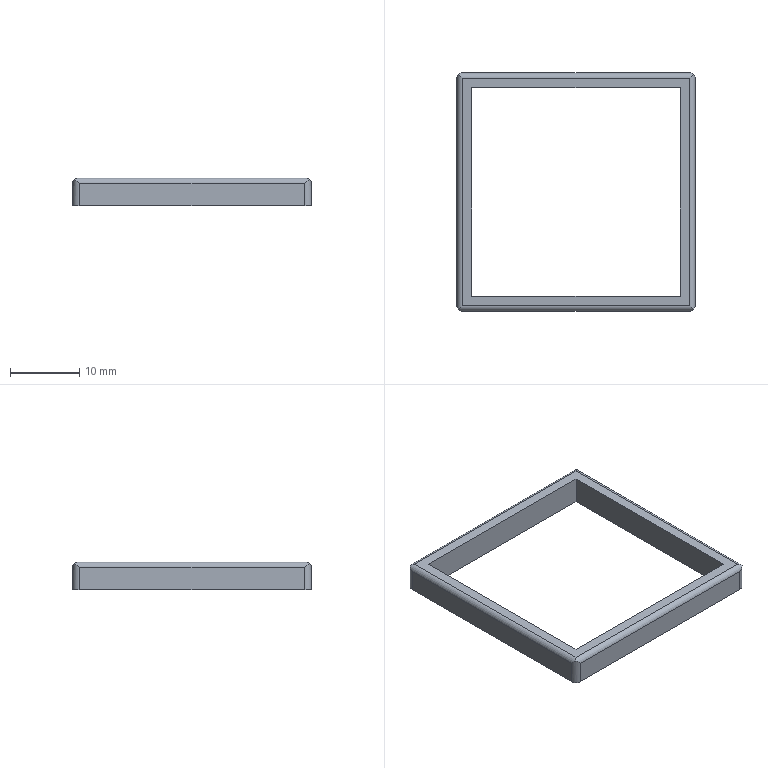Part | NX | 1 solid | 18 faces | box 34.5 x 34.5 x 4 mm | volume 1113 mm3 | plane 10 | cylinder 8 | commonest cylinder face diameters 1.6 x4 2 x4
STEP:
#1=CARTESIAN_POINT('',(16.45,-16.45,21.8));
#2=VERTEX_POINT('',#1);
#3=CARTESIAN_POINT('',(16.957,-16.957,21.619));
#4=VERTEX_POINT('',#3);
#5=CARTESIAN_POINT('',(16.45,-16.45,21.));
#6=DIRECTION('',(-0.7071,-0.7071,0.));
#7=DIRECTION('',(-0.7071,0.7071,0.));
#8=AXIS2_PLACEMENT_3D('',#5,#6,#7);
#9=ELLIPSE('',#8,1.131,0.8);
#10=EDGE_CURVE('',#2,#4,#9,.F.);
#11=ORIENTED_EDGE('',*,*,#10,.F.);
#12=CARTESIAN_POINT('',(-16.45,-16.45,21.8));
#13=VERTEX_POINT('',#12);
#14=CARTESIAN_POINT('',(17.25,-16.45,21.8));
#15=DIRECTION('',(-1.,0.,0.));
#16=VECTOR('',#15,1000.);
#17=LINE('',#14,#16);
#18=EDGE_CURVE('',#2,#13,#17,.T.);
#19=ORIENTED_EDGE('',*,*,#18,.T.);
#20=CARTESIAN_POINT('',(-16.957,-16.957,21.619));
#21=VERTEX_POINT('',#20);
#22=CARTESIAN_POINT('',(-16.45,-16.45,21.));
#23=DIRECTION('',(-0.7071,0.7071,0.));
#24=DIRECTION('',(-0.7071,-0.7071,0.));
#25=AXIS2_PLACEMENT_3D('',#22,#23,#24);
#26=ELLIPSE('',#25,1.131,0.8);
#27=EDGE_CURVE('',#21,#13,#26,.T.);
#28=ORIENTED_EDGE('',*,*,#27,.F.);
#29=CARTESIAN_POINT('',(-16.25,-17.25,21.));
#30=VERTEX_POINT('',#29);
#31=CARTESIAN_POINT('',(-16.957,-16.957,21.619));
#32=CARTESIAN_POINT('',(-16.753,-17.161,21.452));
#33=CARTESIAN_POINT('',(-16.498,-17.25,21.222));
#34=CARTESIAN_POINT('',(-16.25,-17.25,21.));
#35=B_SPLINE_CURVE_WITH_KNOTS('',3,(#31,#32,#33,#34),.UNSPECIFIED.,.F.,.F.,(4,4),(0.0006147,0.001614),.UNSPECIFIED.);
#36=EDGE_CURVE('',#30,#21,#35,.F.);
#37=ORIENTED_EDGE('',*,*,#36,.F.);
#38=CARTESIAN_POINT('',(16.25,-17.25,21.));
#39=VERTEX_POINT('',#38);
#40=CARTESIAN_POINT('',(17.25,-17.25,21.));
#41=DIRECTION('',(-1.,0.,0.));
#42=VECTOR('',#41,1000.);
#43=LINE('',#40,#42);
#44=EDGE_CURVE('',#39,#30,#43,.T.);
#45=ORIENTED_EDGE('',*,*,#44,.F.);
#46=CARTESIAN_POINT('',(16.957,-16.957,21.619));
#47=CARTESIAN_POINT('',(16.753,-17.161,21.452));
#48=CARTESIAN_POINT('',(16.498,-17.25,21.222));
#49=CARTESIAN_POINT('',(16.25,-17.25,21.));
#50=B_SPLINE_CURVE_WITH_KNOTS('',3,(#46,#47,#48,#49),.UNSPECIFIED.,.F.,.F.,(4,4),(0.0006147,0.001614),.UNSPECIFIED.);
#51=EDGE_CURVE('',#4,#39,#50,.T.);
#52=ORIENTED_EDGE('',*,*,#51,.F.);
#53=EDGE_LOOP('',(#11,#19,#28,#37,#45,#52));
#54=FACE_BOUND('',#53,.T.);
#55=CARTESIAN_POINT('',(17.25,-16.45,21.));
#56=DIRECTION('',(-1.,0.,0.));
#57=DIRECTION('',(0.,0.,1.));
#58=AXIS2_PLACEMENT_3D('',#55,#56,#57);
#59=CYLINDRICAL_SURFACE('',#58,0.8);
#60=ADVANCED_FACE('',(#54),#59,.T.);
#61=CARTESIAN_POINT('',(16.957,16.957,21.619));
#62=VERTEX_POINT('',#61);
#63=CARTESIAN_POINT('',(16.45,16.45,21.8));
#64=VERTEX_POINT('',#63);
#65=CARTESIAN_POINT('',(16.45,16.45,21.));
#66=DIRECTION('',(-0.7071,0.7071,0.));
#67=DIRECTION('',(-0.7071,-0.7071,0.));
#68=AXIS2_PLACEMENT_3D('',#65,#66,#67);
#69=ELLIPSE('',#68,1.131,0.8);
#70=EDGE_CURVE('',#62,#64,#69,.F.);
#71=ORIENTED_EDGE('',*,*,#70,.F.);
#72=CARTESIAN_POINT('',(16.25,17.25,21.));
#73=VERTEX_POINT('',#72);
#74=CARTESIAN_POINT('',(16.957,16.957,21.619));
#75=CARTESIAN_POINT('',(16.753,17.161,21.452));
#76=CARTESIAN_POINT('',(16.498,17.25,21.222));
#77=CARTESIAN_POINT('',(16.25,17.25,21.));
#78=B_SPLINE_CURVE_WITH_KNOTS('',3,(#74,#75,#76,#77),.UNSPECIFIED.,.F.,.F.,(4,4),(0.0006147,0.001614),.UNSPECIFIED.);
#79=EDGE_CURVE('',#73,#62,#78,.F.);
#80=ORIENTED_EDGE('',*,*,#79,.F.);
#81=CARTESIAN_POINT('',(-16.25,17.25,21.));
#82=VERTEX_POINT('',#81);
#83=CARTESIAN_POINT('',(17.25,17.25,21.));
#84=DIRECTION('',(-1.,0.,0.));
#85=VECTOR('',#84,1000.);
#86=LINE('',#83,#85);
#87=EDGE_CURVE('',#73,#82,#86,.T.);
#88=ORIENTED_EDGE('',*,*,#87,.T.);
#89=CARTESIAN_POINT('',(-16.957,16.957,21.619));
#90=VERTEX_POINT('',#89);
#91=CARTESIAN_POINT('',(-16.957,16.957,21.619));
#92=CARTESIAN_POINT('',(-16.753,17.161,21.452));
#93=CARTESIAN_POINT('',(-16.498,17.25,21.222));
#94=CARTESIAN_POINT('',(-16.25,17.25,21.));
#95=B_SPLINE_CURVE_WITH_KNOTS('',3,(#91,#92,#93,#94),.UNSPECIFIED.,.F.,.F.,(4,4),(0.0006147,0.001614),.UNSPECIFIED.);
#96=EDGE_CURVE('',#90,#82,#95,.T.);
#97=ORIENTED_EDGE('',*,*,#96,.F.);
#98=CARTESIAN_POINT('',(-16.45,16.45,21.8));
#99=VERTEX_POINT('',#98);
#100=CARTESIAN_POINT('',(-16.45,16.45,21.));
#101=DIRECTION('',(-0.7071,-0.7071,0.));
#102=DIRECTION('',(-0.7071,0.7071,0.));
#103=AXIS2_PLACEMENT_3D('',#100,#101,#102);
#104=ELLIPSE('',#103,1.131,0.8);
#105=EDGE_CURVE('',#99,#90,#104,.T.);
#106=ORIENTED_EDGE('',*,*,#105,.F.);
#107=CARTESIAN_POINT('',(17.25,16.45,21.8));
#108=DIRECTION('',(-1.,0.,0.));
#109=VECTOR('',#108,1000.);
#110=LINE('',#107,#109);
#111=EDGE_CURVE('',#64,#99,#110,.T.);
#112=ORIENTED_EDGE('',*,*,#111,.F.);
#113=EDGE_LOOP('',(#71,#80,#88,#97,#106,#112));
#114=FACE_BOUND('',#113,.T.);
#115=CARTESIAN_POINT('',(17.25,16.45,21.));
#116=DIRECTION('',(-1.,0.,0.));
#117=DIRECTION('',(0.,0.,1.));
#118=AXIS2_PLACEMENT_3D('',#115,#116,#117);
#119=CYLINDRICAL_SURFACE('',#118,0.8);
#120=ADVANCED_FACE('',(#114),#119,.T.);
#121=CARTESIAN_POINT('',(-15.05,-15.05,21.8));
#122=VERTEX_POINT('',#121);
#123=CARTESIAN_POINT('',(-15.05,15.05,21.8));
#124=VERTEX_POINT('',#123);
#125=CARTESIAN_POINT('',(-15.05,16.45,21.8));
#126=DIRECTION('',(0.,1.,0.));
#127=VECTOR('',#126,1000.);
#128=LINE('',#125,#127);
#129=EDGE_CURVE('',#122,#124,#128,.T.);
#130=ORIENTED_EDGE('',*,*,#129,.T.);
#131=CARTESIAN_POINT('',(15.05,15.05,21.8));
#132=VERTEX_POINT('',#131);
#133=CARTESIAN_POINT('',(17.25,15.05,21.8));
#134=DIRECTION('',(1.,0.,0.));
#135=VECTOR('',#134,1000.);
#136=LINE('',#133,#135);
#137=EDGE_CURVE('',#124,#132,#136,.T.);
#138=ORIENTED_EDGE('',*,*,#137,.T.);
#139=CARTESIAN_POINT('',(15.05,-15.05,21.8));
#140=VERTEX_POINT('',#139);
#141=CARTESIAN_POINT('',(15.05,16.45,21.8));
#142=DIRECTION('',(0.,-1.,0.));
#143=VECTOR('',#142,1000.);
#144=LINE('',#141,#143);
#145=EDGE_CURVE('',#132,#140,#144,.T.);
#146=ORIENTED_EDGE('',*,*,#145,.T.);
#147=CARTESIAN_POINT('',(17.25,-15.05,21.8));
#148=DIRECTION('',(-1.,0.,0.));
#149=VECTOR('',#148,1000.);
#150=LINE('',#147,#149);
#151=EDGE_CURVE('',#140,#122,#150,.T.);
#152=ORIENTED_EDGE('',*,*,#151,.T.);
#153=EDGE_LOOP('',(#130,#138,#146,#152));
#154=FACE_BOUND('',#153,.T.);
#155=ORIENTED_EDGE('',*,*,#18,.F.);
#156=CARTESIAN_POINT('',(16.45,-17.25,21.8));
#157=DIRECTION('',(0.,1.,0.));
#158=VECTOR('',#157,1000.);
#159=LINE('',#156,#158);
#160=EDGE_CURVE('',#2,#64,#159,.T.);
#161=ORIENTED_EDGE('',*,*,#160,.T.);
#162=ORIENTED_EDGE('',*,*,#111,.T.);
#163=CARTESIAN_POINT('',(-16.45,-17.25,21.8));
#164=DIRECTION('',(0.,1.,0.));
#165=VECTOR('',#164,1000.);
#166=LINE('',#163,#165);
#167=EDGE_CURVE('',#13,#99,#166,.T.);
#168=ORIENTED_EDGE('',*,*,#167,.F.);
#169=EDGE_LOOP('',(#155,#161,#162,#168));
#170=FACE_BOUND('',#169,.T.);
#171=CARTESIAN_POINT('',(17.25,16.45,21.8));
#172=DIRECTION('',(0.,0.,-1.));
#173=DIRECTION('',(-1.,0.,0.));
#174=AXIS2_PLACEMENT_3D('',#171,#172,#173);
#175=PLANE('',#174);
#176=ADVANCED_FACE('',(#154,#170),#175,.F.);
#177=CARTESIAN_POINT('',(-17.25,16.25,17.8));
#178=VERTEX_POINT('',#177);
#179=CARTESIAN_POINT('',(-17.25,16.25,21.));
#180=VERTEX_POINT('',#179);
#181=CARTESIAN_POINT('',(-17.25,16.25,17.8));
#182=DIRECTION('',(0.,0.,1.));
#183=VECTOR('',#182,1000.);
#184=LINE('',#181,#183);
#185=EDGE_CURVE('',#178,#180,#184,.T.);
#186=ORIENTED_EDGE('',*,*,#185,.T.);
#187=CARTESIAN_POINT('',(-16.957,16.957,21.619));
#188=CARTESIAN_POINT('',(-17.161,16.753,21.452));
#189=CARTESIAN_POINT('',(-17.25,16.498,21.222));
#190=CARTESIAN_POINT('',(-17.25,16.25,21.));
#191=B_SPLINE_CURVE_WITH_KNOTS('',3,(#187,#188,#189,#190),.UNSPECIFIED.,.F.,.F.,(4,4),(0.0006147,0.001614),.UNSPECIFIED.);
#192=EDGE_CURVE('',#180,#90,#191,.F.);
#193=ORIENTED_EDGE('',*,*,#192,.T.);
#194=ORIENTED_EDGE('',*,*,#96,.T.);
#195=CARTESIAN_POINT('',(-16.25,17.25,17.8));
#196=VERTEX_POINT('',#195);
#197=CARTESIAN_POINT('',(-16.25,17.25,17.8));
#198=DIRECTION('',(0.,0.,1.));
#199=VECTOR('',#198,1000.);
#200=LINE('',#197,#199);
#201=EDGE_CURVE('',#196,#82,#200,.T.);
#202=ORIENTED_EDGE('',*,*,#201,.F.);
#203=CARTESIAN_POINT('',(-16.25,16.25,17.8));
#204=DIRECTION('',(0.,0.,1.));
#205=DIRECTION('',(1.,0.,0.));
#206=AXIS2_PLACEMENT_3D('',#203,#204,#205);
#207=CIRCLE('',#206,1.);
#208=EDGE_CURVE('',#196,#178,#207,.T.);
#209=ORIENTED_EDGE('',*,*,#208,.T.);
#210=EDGE_LOOP('',(#186,#193,#194,#202,#209));
#211=FACE_BOUND('',#210,.T.);
#212=CARTESIAN_POINT('',(-16.25,16.25,17.8));
#213=DIRECTION('',(0.,0.,1.));
#214=DIRECTION('',(1.,0.,0.));
#215=AXIS2_PLACEMENT_3D('',#212,#213,#214);
#216=CYLINDRICAL_SURFACE('',#215,1.);
#217=ADVANCED_FACE('',(#211),#216,.T.);
#218=ORIENTED_EDGE('',*,*,#36,.T.);
#219=CARTESIAN_POINT('',(-17.25,-16.25,21.));
#220=VERTEX_POINT('',#219);
#221=CARTESIAN_POINT('',(-16.957,-16.957,21.619));
#222=CARTESIAN_POINT('',(-17.161,-16.753,21.452));
#223=CARTESIAN_POINT('',(-17.25,-16.498,21.222));
#224=CARTESIAN_POINT('',(-17.25,-16.25,21.));
#225=B_SPLINE_CURVE_WITH_KNOTS('',3,(#221,#222,#223,#224),.UNSPECIFIED.,.F.,.F.,(4,4),(0.0006147,0.001614),.UNSPECIFIED.);
#226=EDGE_CURVE('',#21,#220,#225,.T.);
#227=ORIENTED_EDGE('',*,*,#226,.T.);
#228=CARTESIAN_POINT('',(-17.25,-16.25,17.8));
#229=VERTEX_POINT('',#228);
#230=CARTESIAN_POINT('',(-17.25,-16.25,17.8));
#231=DIRECTION('',(0.,0.,1.));
#232=VECTOR('',#231,1000.);
#233=LINE('',#230,#232);
#234=EDGE_CURVE('',#229,#220,#233,.T.);
#235=ORIENTED_EDGE('',*,*,#234,.F.);
#236=CARTESIAN_POINT('',(-16.25,-17.25,17.8));
#237=VERTEX_POINT('',#236);
#238=CARTESIAN_POINT('',(-16.25,-16.25,17.8));
#239=DIRECTION('',(0.,0.,1.));
#240=DIRECTION('',(1.,0.,0.));
#241=AXIS2_PLACEMENT_3D('',#238,#239,#240);
#242=CIRCLE('',#241,1.);
#243=EDGE_CURVE('',#229,#237,#242,.T.);
#244=ORIENTED_EDGE('',*,*,#243,.T.);
#245=CARTESIAN_POINT('',(-16.25,-17.25,17.8));
#246=DIRECTION('',(0.,0.,1.));
#247=VECTOR('',#246,1000.);
#248=LINE('',#245,#247);
#249=EDGE_CURVE('',#237,#30,#248,.T.);
#250=ORIENTED_EDGE('',*,*,#249,.T.);
#251=EDGE_LOOP('',(#218,#227,#235,#244,#250));
#252=FACE_BOUND('',#251,.T.);
#253=CARTESIAN_POINT('',(-16.25,-16.25,17.8));
#254=DIRECTION('',(0.,0.,1.));
#255=DIRECTION('',(1.,0.,0.));
#256=AXIS2_PLACEMENT_3D('',#253,#254,#255);
#257=CYLINDRICAL_SURFACE('',#256,1.);
#258=ADVANCED_FACE('',(#252),#257,.T.);
#259=CARTESIAN_POINT('',(17.25,-16.25,17.8));
#260=VERTEX_POINT('',#259);
#261=CARTESIAN_POINT('',(17.25,-16.25,21.));
#262=VERTEX_POINT('',#261);
#263=CARTESIAN_POINT('',(17.25,-16.25,17.8));
#264=DIRECTION('',(0.,0.,1.));
#265=VECTOR('',#264,1000.);
#266=LINE('',#263,#265);
#267=EDGE_CURVE('',#260,#262,#266,.T.);
#268=ORIENTED_EDGE('',*,*,#267,.T.);
#269=CARTESIAN_POINT('',(16.957,-16.957,21.619));
#270=CARTESIAN_POINT('',(17.161,-16.753,21.452));
#271=CARTESIAN_POINT('',(17.25,-16.498,21.222));
#272=CARTESIAN_POINT('',(17.25,-16.25,21.));
#273=B_SPLINE_CURVE_WITH_KNOTS('',3,(#269,#270,#271,#272),.UNSPECIFIED.,.F.,.F.,(4,4),(0.0006147,0.001614),.UNSPECIFIED.);
#274=EDGE_CURVE('',#262,#4,#273,.F.);
#275=ORIENTED_EDGE('',*,*,#274,.T.);
#276=ORIENTED_EDGE('',*,*,#51,.T.);
#277=CARTESIAN_POINT('',(16.25,-17.25,17.8));
#278=VERTEX_POINT('',#277);
#279=CARTESIAN_POINT('',(16.25,-17.25,17.8));
#280=DIRECTION('',(0.,0.,1.));
#281=VECTOR('',#280,1000.);
#282=LINE('',#279,#281);
#283=EDGE_CURVE('',#278,#39,#282,.T.);
#284=ORIENTED_EDGE('',*,*,#283,.F.);
#285=CARTESIAN_POINT('',(16.25,-16.25,17.8));
#286=DIRECTION('',(0.,0.,1.));
#287=DIRECTION('',(1.,0.,0.));
#288=AXIS2_PLACEMENT_3D('',#285,#286,#287);
#289=CIRCLE('',#288,1.);
#290=EDGE_CURVE('',#278,#260,#289,.T.);
#291=ORIENTED_EDGE('',*,*,#290,.T.);
#292=EDGE_LOOP('',(#268,#275,#276,#284,#291));
#293=FACE_BOUND('',#292,.T.);
#294=CARTESIAN_POINT('',(16.25,-16.25,17.8));
#295=DIRECTION('',(0.,0.,1.));
#296=DIRECTION('',(1.,0.,0.));
#297=AXIS2_PLACEMENT_3D('',#294,#295,#296);
#298=CYLINDRICAL_SURFACE('',#297,1.);
#299=ADVANCED_FACE('',(#293),#298,.T.);
#300=ORIENTED_EDGE('',*,*,#79,.T.);
#301=CARTESIAN_POINT('',(17.25,16.25,21.));
#302=VERTEX_POINT('',#301);
#303=CARTESIAN_POINT('',(16.957,16.957,21.619));
#304=CARTESIAN_POINT('',(17.161,16.753,21.452));
#305=CARTESIAN_POINT('',(17.25,16.498,21.222));
#306=CARTESIAN_POINT('',(17.25,16.25,21.));
#307=B_SPLINE_CURVE_WITH_KNOTS('',3,(#303,#304,#305,#306),.UNSPECIFIED.,.F.,.F.,(4,4),(0.0006147,0.001614),.UNSPECIFIED.);
#308=EDGE_CURVE('',#62,#302,#307,.T.);
#309=ORIENTED_EDGE('',*,*,#308,.T.);
#310=CARTESIAN_POINT('',(17.25,16.25,17.8));
#311=VERTEX_POINT('',#310);
#312=CARTESIAN_POINT('',(17.25,16.25,17.8));
#313=DIRECTION('',(0.,0.,1.));
#314=VECTOR('',#313,1000.);
#315=LINE('',#312,#314);
#316=EDGE_CURVE('',#311,#302,#315,.T.);
#317=ORIENTED_EDGE('',*,*,#316,.F.);
#318=CARTESIAN_POINT('',(16.25,17.25,17.8));
#319=VERTEX_POINT('',#318);
#320=CARTESIAN_POINT('',(16.25,16.25,17.8));
#321=DIRECTION('',(0.,0.,1.));
#322=DIRECTION('',(1.,0.,0.));
#323=AXIS2_PLACEMENT_3D('',#320,#321,#322);
#324=CIRCLE('',#323,1.);
#325=EDGE_CURVE('',#311,#319,#324,.T.);
#326=ORIENTED_EDGE('',*,*,#325,.T.);
#327=CARTESIAN_POINT('',(16.25,17.25,17.8));
#328=DIRECTION('',(0.,0.,1.));
#329=VECTOR('',#328,1000.);
#330=LINE('',#327,#329);
#331=EDGE_CURVE('',#319,#73,#330,.T.);
#332=ORIENTED_EDGE('',*,*,#331,.T.);
#333=EDGE_LOOP('',(#300,#309,#317,#326,#332));
#334=FACE_BOUND('',#333,.T.);
#335=CARTESIAN_POINT('',(16.25,16.25,17.8));
#336=DIRECTION('',(0.,0.,1.));
#337=DIRECTION('',(1.,0.,0.));
#338=AXIS2_PLACEMENT_3D('',#335,#336,#337);
#339=CYLINDRICAL_SURFACE('',#338,1.);
#340=ADVANCED_FACE('',(#334),#339,.T.);
#341=ORIENTED_EDGE('',*,*,#249,.F.);
#342=CARTESIAN_POINT('',(17.25,-17.25,17.8));
#343=DIRECTION('',(-1.,0.,0.));
#344=VECTOR('',#343,1000.);
#345=LINE('',#342,#344);
#346=EDGE_CURVE('',#278,#237,#345,.T.);
#347=ORIENTED_EDGE('',*,*,#346,.F.);
#348=ORIENTED_EDGE('',*,*,#283,.T.);
#349=ORIENTED_EDGE('',*,*,#44,.T.);
#350=EDGE_LOOP('',(#341,#347,#348,#349));
#351=FACE_BOUND('',#350,.T.);
#352=CARTESIAN_POINT('',(17.25,-17.25,21.));
#353=DIRECTION('',(0.,1.,0.));
#354=DIRECTION('',(0.,0.,1.));
#355=AXIS2_PLACEMENT_3D('',#352,#353,#354);
#356=PLANE('',#355);
#357=ADVANCED_FACE('',(#351),#356,.F.);
#358=CARTESIAN_POINT('',(15.05,-15.05,17.8));
#359=VERTEX_POINT('',#358);
#360=CARTESIAN_POINT('',(15.05,15.05,17.8));
#361=VERTEX_POINT('',#360);
#362=CARTESIAN_POINT('',(15.05,-15.05,17.8));
#363=DIRECTION('',(0.,1.,0.));
#364=VECTOR('',#363,1000.);
#365=LINE('',#362,#364);
#366=EDGE_CURVE('',#359,#361,#365,.T.);
#367=ORIENTED_EDGE('',*,*,#366,.T.);
#368=CARTESIAN_POINT('',(-15.05,15.05,17.8));
#369=VERTEX_POINT('',#368);
#370=CARTESIAN_POINT('',(15.05,15.05,17.8));
#371=DIRECTION('',(-1.,0.,0.));
#372=VECTOR('',#371,1000.);
#373=LINE('',#370,#372);
#374=EDGE_CURVE('',#361,#369,#373,.T.);
#375=ORIENTED_EDGE('',*,*,#374,.T.);
#376=CARTESIAN_POINT('',(-15.05,-15.05,17.8));
#377=VERTEX_POINT('',#376);
#378=CARTESIAN_POINT('',(-15.05,15.05,17.8));
#379=DIRECTION('',(0.,-1.,0.));
#380=VECTOR('',#379,1000.);
#381=LINE('',#378,#380);
#382=EDGE_CURVE('',#369,#377,#381,.T.);
#383=ORIENTED_EDGE('',*,*,#382,.T.);
#384=CARTESIAN_POINT('',(-15.05,-15.05,17.8));
#385=DIRECTION('',(1.,0.,0.));
#386=VECTOR('',#385,1000.);
#387=LINE('',#384,#386);
#388=EDGE_CURVE('',#377,#359,#387,.T.);
#389=ORIENTED_EDGE('',*,*,#388,.T.);
#390=EDGE_LOOP('',(#367,#375,#383,#389));
#391=FACE_BOUND('',#390,.T.);
#392=ORIENTED_EDGE('',*,*,#243,.F.);
#393=CARTESIAN_POINT('',(-17.25,-17.25,17.8));
#394=DIRECTION('',(0.,1.,0.));
#395=VECTOR('',#394,1000.);
#396=LINE('',#393,#395);
#397=EDGE_CURVE('',#229,#178,#396,.T.);
#398=ORIENTED_EDGE('',*,*,#397,.T.);
#399=ORIENTED_EDGE('',*,*,#208,.F.);
#400=CARTESIAN_POINT('',(17.25,17.25,17.8));
#401=DIRECTION('',(-1.,0.,0.));
#402=VECTOR('',#401,1000.);
#403=LINE('',#400,#402);
#404=EDGE_CURVE('',#319,#196,#403,.T.);
#405=ORIENTED_EDGE('',*,*,#404,.F.);
#406=ORIENTED_EDGE('',*,*,#325,.F.);
#407=CARTESIAN_POINT('',(17.25,-17.25,17.8));
#408=DIRECTION('',(0.,1.,0.));
#409=VECTOR('',#408,1000.);
#410=LINE('',#407,#409);
#411=EDGE_CURVE('',#260,#311,#410,.T.);
#412=ORIENTED_EDGE('',*,*,#411,.F.);
#413=ORIENTED_EDGE('',*,*,#290,.F.);
#414=ORIENTED_EDGE('',*,*,#346,.T.);
#415=EDGE_LOOP('',(#392,#398,#399,#405,#406,#412,#413,#414));
#416=FACE_BOUND('',#415,.T.);
#417=CARTESIAN_POINT('',(17.25,-17.25,17.8));
#418=DIRECTION('',(0.,0.,1.));
#419=DIRECTION('',(1.,0.,0.));
#420=AXIS2_PLACEMENT_3D('',#417,#418,#419);
#421=PLANE('',#420);
#422=ADVANCED_FACE('',(#391,#416),#421,.F.);
#423=ORIENTED_EDGE('',*,*,#404,.T.);
#424=ORIENTED_EDGE('',*,*,#201,.T.);
#425=ORIENTED_EDGE('',*,*,#87,.F.);
#426=ORIENTED_EDGE('',*,*,#331,.F.);
#427=EDGE_LOOP('',(#423,#424,#425,#426));
#428=FACE_BOUND('',#427,.T.);
#429=CARTESIAN_POINT('',(17.25,17.25,17.8));
#430=DIRECTION('',(0.,-1.,0.));
#431=DIRECTION('',(0.,0.,-1.));
#432=AXIS2_PLACEMENT_3D('',#429,#430,#431);
#433=PLANE('',#432);
#434=ADVANCED_FACE('',(#428),#433,.F.);
#435=CARTESIAN_POINT('',(17.25,-17.25,21.));
#436=DIRECTION('',(0.,1.,0.));
#437=VECTOR('',#436,1000.);
#438=LINE('',#435,#437);
#439=EDGE_CURVE('',#262,#302,#438,.T.);
#440=ORIENTED_EDGE('',*,*,#439,.F.);
#441=ORIENTED_EDGE('',*,*,#267,.F.);
#442=ORIENTED_EDGE('',*,*,#411,.T.);
#443=ORIENTED_EDGE('',*,*,#316,.T.);
#444=EDGE_LOOP('',(#440,#441,#442,#443));
#445=FACE_BOUND('',#444,.T.);
#446=CARTESIAN_POINT('',(17.25,-16.45,21.));
#447=DIRECTION('',(1.,0.,0.));
#448=DIRECTION('',(0.,0.,-1.));
#449=AXIS2_PLACEMENT_3D('',#446,#447,#448);
#450=PLANE('',#449);
#451=ADVANCED_FACE('',(#445),#450,.T.);
#452=ORIENTED_EDGE('',*,*,#234,.T.);
#453=CARTESIAN_POINT('',(-17.25,-17.25,21.));
#454=DIRECTION('',(0.,1.,0.));
#455=VECTOR('',#454,1000.);
#456=LINE('',#453,#455);
#457=EDGE_CURVE('',#220,#180,#456,.T.);
#458=ORIENTED_EDGE('',*,*,#457,.T.);
#459=ORIENTED_EDGE('',*,*,#185,.F.);
#460=ORIENTED_EDGE('',*,*,#397,.F.);
#461=EDGE_LOOP('',(#452,#458,#459,#460));
#462=FACE_BOUND('',#461,.T.);
#463=CARTESIAN_POINT('',(-17.25,-16.45,21.));
#464=DIRECTION('',(1.,0.,0.));
#465=DIRECTION('',(0.,0.,-1.));
#466=AXIS2_PLACEMENT_3D('',#463,#464,#465);
#467=PLANE('',#466);
#468=ADVANCED_FACE('',(#462),#467,.F.);
#469=ORIENTED_EDGE('',*,*,#10,.T.);
#470=ORIENTED_EDGE('',*,*,#274,.F.);
#471=ORIENTED_EDGE('',*,*,#439,.T.);
#472=ORIENTED_EDGE('',*,*,#308,.F.);
#473=ORIENTED_EDGE('',*,*,#70,.T.);
#474=ORIENTED_EDGE('',*,*,#160,.F.);
#475=EDGE_LOOP('',(#469,#470,#471,#472,#473,#474));
#476=FACE_BOUND('',#475,.T.);
#477=CARTESIAN_POINT('',(16.45,-17.25,21.));
#478=DIRECTION('',(0.,1.,0.));
#479=DIRECTION('',(0.,0.,1.));
#480=AXIS2_PLACEMENT_3D('',#477,#478,#479);
#481=CYLINDRICAL_SURFACE('',#480,0.8);
#482=ADVANCED_FACE('',(#476),#481,.T.);
#483=ORIENTED_EDGE('',*,*,#105,.T.);
#484=ORIENTED_EDGE('',*,*,#192,.F.);
#485=ORIENTED_EDGE('',*,*,#457,.F.);
#486=ORIENTED_EDGE('',*,*,#226,.F.);
#487=ORIENTED_EDGE('',*,*,#27,.T.);
#488=ORIENTED_EDGE('',*,*,#167,.T.);
#489=EDGE_LOOP('',(#483,#484,#485,#486,#487,#488));
#490=FACE_BOUND('',#489,.T.);
#491=CARTESIAN_POINT('',(-16.45,-17.25,21.));
#492=DIRECTION('',(0.,1.,0.));
#493=DIRECTION('',(0.,0.,1.));
#494=AXIS2_PLACEMENT_3D('',#491,#492,#493);
#495=CYLINDRICAL_SURFACE('',#494,0.8);
#496=ADVANCED_FACE('',(#490),#495,.T.);
#497=CARTESIAN_POINT('',(-15.05,15.05,17.8));
#498=DIRECTION('',(0.,0.,1.));
#499=VECTOR('',#498,1000.);
#500=LINE('',#497,#499);
#501=EDGE_CURVE('',#369,#124,#500,.T.);
#502=ORIENTED_EDGE('',*,*,#501,.F.);
#503=ORIENTED_EDGE('',*,*,#374,.F.);
#504=CARTESIAN_POINT('',(15.05,15.05,17.8));
#505=DIRECTION('',(0.,0.,1.));
#506=VECTOR('',#505,1000.);
#507=LINE('',#504,#506);
#508=EDGE_CURVE('',#361,#132,#507,.T.);
#509=ORIENTED_EDGE('',*,*,#508,.T.);
#510=ORIENTED_EDGE('',*,*,#137,.F.);
#511=EDGE_LOOP('',(#502,#503,#509,#510));
#512=FACE_BOUND('',#511,.T.);
#513=CARTESIAN_POINT('',(15.05,15.05,17.8));
#514=DIRECTION('',(0.,1.,0.));
#515=DIRECTION('',(0.,0.,1.));
#516=AXIS2_PLACEMENT_3D('',#513,#514,#515);
#517=PLANE('',#516);
#518=ADVANCED_FACE('',(#512),#517,.F.);
#519=ORIENTED_EDGE('',*,*,#508,.F.);
#520=ORIENTED_EDGE('',*,*,#366,.F.);
#521=CARTESIAN_POINT('',(15.05,-15.05,17.8));
#522=DIRECTION('',(0.,0.,1.));
#523=VECTOR('',#522,1000.);
#524=LINE('',#521,#523);
#525=EDGE_CURVE('',#359,#140,#524,.T.);
#526=ORIENTED_EDGE('',*,*,#525,.T.);
#527=ORIENTED_EDGE('',*,*,#145,.F.);
#528=EDGE_LOOP('',(#519,#520,#526,#527));
#529=FACE_BOUND('',#528,.T.);
#530=CARTESIAN_POINT('',(15.05,-15.05,17.8));
#531=DIRECTION('',(1.,0.,0.));
#532=DIRECTION('',(0.,1.,0.));
#533=AXIS2_PLACEMENT_3D('',#530,#531,#532);
#534=PLANE('',#533);
#535=ADVANCED_FACE('',(#529),#534,.F.);
#536=ORIENTED_EDGE('',*,*,#525,.F.);
#537=ORIENTED_EDGE('',*,*,#388,.F.);
#538=CARTESIAN_POINT('',(-15.05,-15.05,17.8));
#539=DIRECTION('',(0.,0.,1.));
#540=VECTOR('',#539,1000.);
#541=LINE('',#538,#540);
#542=EDGE_CURVE('',#377,#122,#541,.T.);
#543=ORIENTED_EDGE('',*,*,#542,.T.);
#544=ORIENTED_EDGE('',*,*,#151,.F.);
#545=EDGE_LOOP('',(#536,#537,#543,#544));
#546=FACE_BOUND('',#545,.T.);
#547=CARTESIAN_POINT('',(-15.05,-15.05,17.8));
#548=DIRECTION('',(0.,-1.,0.));
#549=DIRECTION('',(0.,0.,-1.));
#550=AXIS2_PLACEMENT_3D('',#547,#548,#549);
#551=PLANE('',#550);
#552=ADVANCED_FACE('',(#546),#551,.F.);
#553=ORIENTED_EDGE('',*,*,#542,.F.);
#554=ORIENTED_EDGE('',*,*,#382,.F.);
#555=ORIENTED_EDGE('',*,*,#501,.T.);
#556=ORIENTED_EDGE('',*,*,#129,.F.);
#557=EDGE_LOOP('',(#553,#554,#555,#556));
#558=FACE_BOUND('',#557,.T.);
#559=CARTESIAN_POINT('',(-15.05,15.05,17.8));
#560=DIRECTION('',(-1.,0.,0.));
#561=DIRECTION('',(0.,0.,1.));
#562=AXIS2_PLACEMENT_3D('',#559,#560,#561);
#563=PLANE('',#562);
#564=ADVANCED_FACE('',(#558),#563,.F.);
#565=CLOSED_SHELL('',(#60,#120,#176,#217,#258,#299,#340,#357,#422,#434,#451,#468,#482,#496,#518,#535,#552,#564));
#566=MANIFOLD_SOLID_BREP('',#565);
#567=(LENGTH_UNIT()NAMED_UNIT(*)SI_UNIT(.MILLI.,.METRE.));
#568=UNCERTAINTY_MEASURE_WITH_UNIT(LENGTH_MEASURE(0.0508),#567,'','');
#569=(NAMED_UNIT(*)PLANE_ANGLE_UNIT()SI_UNIT($,.RADIAN.));
#570=(NAMED_UNIT(*)SI_UNIT($,.STERADIAN.)SOLID_ANGLE_UNIT());
#571=(GEOMETRIC_REPRESENTATION_CONTEXT(3)GLOBAL_UNCERTAINTY_ASSIGNED_CONTEXT((#568))GLOBAL_UNIT_ASSIGNED_CONTEXT((#567,#569,#570))REPRESENTATION_CONTEXT('',''));
#572=ADVANCED_BREP_SHAPE_REPRESENTATION('',(#566),#571);